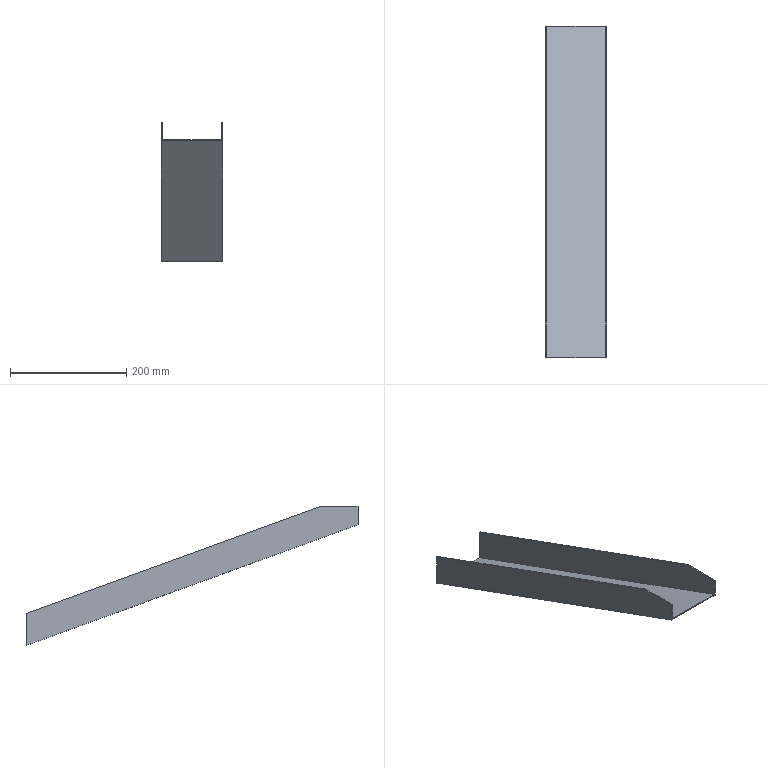Part | NX | features solid 2 | 1 solid | 12 faces | box 105.075 x 570 x 238.942 mm | volume 245403 mm3 | plane 12
STEP:
#1=CARTESIAN_POINT('',(52.538,10.,-231.479));
#2=VERTEX_POINT('',#1);
#3=CARTESIAN_POINT('',(52.538,10.,-200.));
#4=VERTEX_POINT('',#3);
#5=CARTESIAN_POINT('',(52.538,10.,-230.));
#6=DIRECTION('',(0.,0.,1.));
#7=VECTOR('',#6,1000.);
#8=LINE('',#5,#7);
#9=EDGE_CURVE('',#2,#4,#8,.T.);
#10=ORIENTED_EDGE('',*,*,#9,.F.);
#11=CARTESIAN_POINT('',(52.538,580.,-438.942));
#12=VERTEX_POINT('',#11);
#13=CARTESIAN_POINT('',(52.538,11.431,-232.));
#14=DIRECTION('',(0.,-0.9397,0.342));
#15=VECTOR('',#14,1000.);
#16=LINE('',#13,#15);
#17=EDGE_CURVE('',#2,#12,#16,.F.);
#18=ORIENTED_EDGE('',*,*,#17,.T.);
#19=CARTESIAN_POINT('',(52.538,580.,-383.733));
#20=VERTEX_POINT('',#19);
#21=CARTESIAN_POINT('',(52.538,580.,-230.));
#22=DIRECTION('',(0.,0.,1.));
#23=VECTOR('',#22,1000.);
#24=LINE('',#21,#23);
#25=EDGE_CURVE('',#12,#20,#24,.T.);
#26=ORIENTED_EDGE('',*,*,#25,.T.);
#27=CARTESIAN_POINT('',(52.538,75.196,-200.));
#28=VERTEX_POINT('',#27);
#29=CARTESIAN_POINT('',(52.538,28.532,-183.015));
#30=DIRECTION('',(0.,0.9397,-0.342));
#31=VECTOR('',#30,1000.);
#32=LINE('',#29,#31);
#33=EDGE_CURVE('',#28,#20,#32,.T.);
#34=ORIENTED_EDGE('',*,*,#33,.F.);
#35=CARTESIAN_POINT('',(52.538,380.,-200.));
#36=DIRECTION('',(0.,-1.,0.));
#37=VECTOR('',#36,1000.);
#38=LINE('',#35,#37);
#39=EDGE_CURVE('',#28,#4,#38,.T.);
#40=ORIENTED_EDGE('',*,*,#39,.T.);
#41=EDGE_LOOP('',(#10,#18,#26,#34,#40));
#42=FACE_BOUND('',#41,.T.);
#43=CARTESIAN_POINT('',(52.538,11.431,-230.));
#44=DIRECTION('',(-1.,0.,0.));
#45=DIRECTION('',(0.,0.,-1.));
#46=AXIS2_PLACEMENT_3D('',#43,#44,#45);
#47=PLANE('',#46);
#48=ADVANCED_FACE('',(#42),#47,.F.);
#49=CARTESIAN_POINT('',(50.538,10.,-200.));
#50=VERTEX_POINT('',#49);
#51=CARTESIAN_POINT('',(50.538,10.,-229.351));
#52=VERTEX_POINT('',#51);
#53=CARTESIAN_POINT('',(50.538,10.,-183.015));
#54=DIRECTION('',(0.,0.,-1.));
#55=VECTOR('',#54,1000.);
#56=LINE('',#53,#55);
#57=EDGE_CURVE('',#50,#52,#56,.T.);
#58=ORIENTED_EDGE('',*,*,#57,.F.);
#59=CARTESIAN_POINT('',(50.538,75.196,-200.));
#60=VERTEX_POINT('',#59);
#61=CARTESIAN_POINT('',(50.538,380.,-200.));
#62=DIRECTION('',(0.,1.,0.));
#63=VECTOR('',#62,1000.);
#64=LINE('',#61,#63);
#65=EDGE_CURVE('',#50,#60,#64,.T.);
#66=ORIENTED_EDGE('',*,*,#65,.T.);
#67=CARTESIAN_POINT('',(50.538,580.,-383.733));
#68=VERTEX_POINT('',#67);
#69=CARTESIAN_POINT('',(50.538,28.532,-183.015));
#70=DIRECTION('',(0.,0.9397,-0.342));
#71=VECTOR('',#70,1000.);
#72=LINE('',#69,#71);
#73=EDGE_CURVE('',#60,#68,#72,.T.);
#74=ORIENTED_EDGE('',*,*,#73,.T.);
#75=CARTESIAN_POINT('',(50.538,580.,-436.814));
#76=VERTEX_POINT('',#75);
#77=CARTESIAN_POINT('',(50.538,580.,-183.015));
#78=DIRECTION('',(0.,0.,-1.));
#79=VECTOR('',#78,1000.);
#80=LINE('',#77,#79);
#81=EDGE_CURVE('',#68,#76,#80,.T.);
#82=ORIENTED_EDGE('',*,*,#81,.T.);
#83=CARTESIAN_POINT('',(50.538,12.115,-230.121));
#84=DIRECTION('',(0.,-0.9397,0.342));
#85=VECTOR('',#84,1000.);
#86=LINE('',#83,#85);
#87=EDGE_CURVE('',#52,#76,#86,.F.);
#88=ORIENTED_EDGE('',*,*,#87,.F.);
#89=EDGE_LOOP('',(#58,#66,#74,#82,#88));
#90=FACE_BOUND('',#89,.T.);
#91=CARTESIAN_POINT('',(50.538,28.532,-183.015));
#92=DIRECTION('',(1.,0.,0.));
#93=DIRECTION('',(0.,0.,1.));
#94=AXIS2_PLACEMENT_3D('',#91,#92,#93);
#95=PLANE('',#94);
#96=ADVANCED_FACE('',(#90),#95,.F.);
#97=CARTESIAN_POINT('',(-50.538,10.,-229.351));
#98=VERTEX_POINT('',#97);
#99=CARTESIAN_POINT('',(42.538,10.,-229.351));
#100=DIRECTION('',(1.,0.,0.));
#101=VECTOR('',#100,1000.);
#102=LINE('',#99,#101);
#103=EDGE_CURVE('',#52,#98,#102,.F.);
#104=ORIENTED_EDGE('',*,*,#103,.F.);
#105=ORIENTED_EDGE('',*,*,#87,.T.);
#106=CARTESIAN_POINT('',(-50.538,580.,-436.814));
#107=VERTEX_POINT('',#106);
#108=CARTESIAN_POINT('',(42.538,580.,-436.814));
#109=DIRECTION('',(1.,0.,0.));
#110=VECTOR('',#109,1000.);
#111=LINE('',#108,#110);
#112=EDGE_CURVE('',#76,#107,#111,.F.);
#113=ORIENTED_EDGE('',*,*,#112,.T.);
#114=CARTESIAN_POINT('',(-50.538,12.115,-230.121));
#115=DIRECTION('',(0.,-0.9397,0.342));
#116=VECTOR('',#115,1000.);
#117=LINE('',#114,#116);
#118=EDGE_CURVE('',#98,#107,#117,.F.);
#119=ORIENTED_EDGE('',*,*,#118,.F.);
#120=EDGE_LOOP('',(#104,#105,#113,#119));
#121=FACE_BOUND('',#120,.T.);
#122=CARTESIAN_POINT('',(42.538,12.115,-230.121));
#123=DIRECTION('',(0.,0.342,0.9397));
#124=DIRECTION('',(0.,0.9397,-0.342));
#125=AXIS2_PLACEMENT_3D('',#122,#123,#124);
#126=PLANE('',#125);
#127=ADVANCED_FACE('',(#121),#126,.T.);
#128=ORIENTED_EDGE('',*,*,#17,.F.);
#129=CARTESIAN_POINT('',(-52.538,10.,-231.479));
#130=VERTEX_POINT('',#129);
#131=CARTESIAN_POINT('',(42.538,10.,-231.479));
#132=DIRECTION('',(1.,0.,0.));
#133=VECTOR('',#132,1000.);
#134=LINE('',#131,#133);
#135=EDGE_CURVE('',#2,#130,#134,.F.);
#136=ORIENTED_EDGE('',*,*,#135,.T.);
#137=CARTESIAN_POINT('',(-52.538,580.,-438.942));
#138=VERTEX_POINT('',#137);
#139=CARTESIAN_POINT('',(-52.538,11.431,-232.));
#140=DIRECTION('',(0.,-0.9397,0.342));
#141=VECTOR('',#140,1000.);
#142=LINE('',#139,#141);
#143=EDGE_CURVE('',#130,#138,#142,.F.);
#144=ORIENTED_EDGE('',*,*,#143,.T.);
#145=CARTESIAN_POINT('',(42.538,580.,-438.942));
#146=DIRECTION('',(1.,0.,0.));
#147=VECTOR('',#146,1000.);
#148=LINE('',#145,#147);
#149=EDGE_CURVE('',#12,#138,#148,.F.);
#150=ORIENTED_EDGE('',*,*,#149,.F.);
#151=EDGE_LOOP('',(#128,#136,#144,#150));
#152=FACE_BOUND('',#151,.T.);
#153=CARTESIAN_POINT('',(42.538,11.431,-232.));
#154=DIRECTION('',(0.,0.342,0.9397));
#155=DIRECTION('',(0.,0.9397,-0.342));
#156=AXIS2_PLACEMENT_3D('',#153,#154,#155);
#157=PLANE('',#156);
#158=ADVANCED_FACE('',(#152),#157,.F.);
#159=ORIENTED_EDGE('',*,*,#65,.F.);
#160=CARTESIAN_POINT('',(-35.,10.,-200.));
#161=DIRECTION('',(1.,0.,0.));
#162=VECTOR('',#161,1000.);
#163=LINE('',#160,#162);
#164=EDGE_CURVE('',#50,#4,#163,.T.);
#165=ORIENTED_EDGE('',*,*,#164,.T.);
#166=ORIENTED_EDGE('',*,*,#39,.F.);
#167=CARTESIAN_POINT('',(-35.,75.196,-200.));
#168=DIRECTION('',(-1.,0.,0.));
#169=VECTOR('',#168,1000.);
#170=LINE('',#167,#169);
#171=EDGE_CURVE('',#28,#60,#170,.T.);
#172=ORIENTED_EDGE('',*,*,#171,.T.);
#173=EDGE_LOOP('',(#159,#165,#166,#172));
#174=FACE_BOUND('',#173,.T.);
#175=CARTESIAN_POINT('',(-35.,380.,-200.));
#176=DIRECTION('',(0.,0.,1.));
#177=DIRECTION('',(-1.,0.,0.));
#178=AXIS2_PLACEMENT_3D('',#175,#176,#177);
#179=PLANE('',#178);
#180=ADVANCED_FACE('',(#174),#179,.T.);
#181=CARTESIAN_POINT('',(-52.538,10.,-200.));
#182=VERTEX_POINT('',#181);
#183=CARTESIAN_POINT('',(-52.538,10.,-230.));
#184=DIRECTION('',(0.,0.,-1.));
#185=VECTOR('',#184,1000.);
#186=LINE('',#183,#185);
#187=EDGE_CURVE('',#182,#130,#186,.T.);
#188=ORIENTED_EDGE('',*,*,#187,.F.);
#189=CARTESIAN_POINT('',(-52.538,75.196,-200.));
#190=VERTEX_POINT('',#189);
#191=CARTESIAN_POINT('',(-52.538,11.431,-200.));
#192=DIRECTION('',(0.,-1.,0.));
#193=VECTOR('',#192,1000.);
#194=LINE('',#191,#193);
#195=EDGE_CURVE('',#190,#182,#194,.T.);
#196=ORIENTED_EDGE('',*,*,#195,.F.);
#197=CARTESIAN_POINT('',(-52.538,580.,-383.733));
#198=VERTEX_POINT('',#197);
#199=CARTESIAN_POINT('',(-52.538,28.532,-183.015));
#200=DIRECTION('',(0.,0.9397,-0.342));
#201=VECTOR('',#200,1000.);
#202=LINE('',#199,#201);
#203=EDGE_CURVE('',#190,#198,#202,.T.);
#204=ORIENTED_EDGE('',*,*,#203,.T.);
#205=CARTESIAN_POINT('',(-52.538,580.,-405.));
#206=DIRECTION('',(0.,0.,1.));
#207=VECTOR('',#206,1000.);
#208=LINE('',#205,#207);
#209=EDGE_CURVE('',#138,#198,#208,.T.);
#210=ORIENTED_EDGE('',*,*,#209,.F.);
#211=ORIENTED_EDGE('',*,*,#143,.F.);
#212=EDGE_LOOP('',(#188,#196,#204,#210,#211));
#213=FACE_BOUND('',#212,.T.);
#214=CARTESIAN_POINT('',(-52.538,11.431,-230.));
#215=DIRECTION('',(1.,0.,0.));
#216=DIRECTION('',(0.,0.,-1.));
#217=AXIS2_PLACEMENT_3D('',#214,#215,#216);
#218=PLANE('',#217);
#219=ADVANCED_FACE('',(#213),#218,.F.);
#220=CARTESIAN_POINT('',(-50.538,10.,-200.));
#221=VERTEX_POINT('',#220);
#222=CARTESIAN_POINT('',(-50.538,10.,-183.015));
#223=DIRECTION('',(0.,0.,1.));
#224=VECTOR('',#223,1000.);
#225=LINE('',#222,#224);
#226=EDGE_CURVE('',#98,#221,#225,.T.);
#227=ORIENTED_EDGE('',*,*,#226,.F.);
#228=ORIENTED_EDGE('',*,*,#118,.T.);
#229=CARTESIAN_POINT('',(-50.538,580.,-383.733));
#230=VERTEX_POINT('',#229);
#231=CARTESIAN_POINT('',(-50.538,580.,-405.));
#232=DIRECTION('',(0.,0.,-1.));
#233=VECTOR('',#232,1000.);
#234=LINE('',#231,#233);
#235=EDGE_CURVE('',#230,#107,#234,.T.);
#236=ORIENTED_EDGE('',*,*,#235,.F.);
#237=CARTESIAN_POINT('',(-50.538,75.196,-200.));
#238=VERTEX_POINT('',#237);
#239=CARTESIAN_POINT('',(-50.538,28.532,-183.015));
#240=DIRECTION('',(0.,0.9397,-0.342));
#241=VECTOR('',#240,1000.);
#242=LINE('',#239,#241);
#243=EDGE_CURVE('',#238,#230,#242,.T.);
#244=ORIENTED_EDGE('',*,*,#243,.F.);
#245=CARTESIAN_POINT('',(-50.538,28.532,-200.));
#246=DIRECTION('',(0.,1.,0.));
#247=VECTOR('',#246,1000.);
#248=LINE('',#245,#247);
#249=EDGE_CURVE('',#221,#238,#248,.T.);
#250=ORIENTED_EDGE('',*,*,#249,.F.);
#251=EDGE_LOOP('',(#227,#228,#236,#244,#250));
#252=FACE_BOUND('',#251,.T.);
#253=CARTESIAN_POINT('',(-50.538,28.532,-183.015));
#254=DIRECTION('',(-1.,0.,0.));
#255=DIRECTION('',(0.,0.,1.));
#256=AXIS2_PLACEMENT_3D('',#253,#254,#255);
#257=PLANE('',#256);
#258=ADVANCED_FACE('',(#252),#257,.F.);
#259=ORIENTED_EDGE('',*,*,#195,.T.);
#260=CARTESIAN_POINT('',(35.,10.,-200.));
#261=DIRECTION('',(1.,0.,0.));
#262=VECTOR('',#261,1000.);
#263=LINE('',#260,#262);
#264=EDGE_CURVE('',#182,#221,#263,.T.);
#265=ORIENTED_EDGE('',*,*,#264,.T.);
#266=ORIENTED_EDGE('',*,*,#249,.T.);
#267=CARTESIAN_POINT('',(-52.538,75.196,-200.));
#268=DIRECTION('',(1.,0.,0.));
#269=VECTOR('',#268,1000.);
#270=LINE('',#267,#269);
#271=EDGE_CURVE('',#190,#238,#270,.T.);
#272=ORIENTED_EDGE('',*,*,#271,.F.);
#273=EDGE_LOOP('',(#259,#265,#266,#272));
#274=FACE_BOUND('',#273,.T.);
#275=CARTESIAN_POINT('',(35.,380.,-200.));
#276=DIRECTION('',(0.,0.,1.));
#277=DIRECTION('',(1.,0.,0.));
#278=AXIS2_PLACEMENT_3D('',#275,#276,#277);
#279=PLANE('',#278);
#280=ADVANCED_FACE('',(#274),#279,.T.);
#281=ORIENTED_EDGE('',*,*,#33,.T.);
#282=CARTESIAN_POINT('',(330.,580.,-383.733));
#283=DIRECTION('',(-1.,0.,0.));
#284=VECTOR('',#283,1000.);
#285=LINE('',#282,#284);
#286=EDGE_CURVE('',#20,#68,#285,.T.);
#287=ORIENTED_EDGE('',*,*,#286,.T.);
#288=ORIENTED_EDGE('',*,*,#73,.F.);
#289=ORIENTED_EDGE('',*,*,#171,.F.);
#290=EDGE_LOOP('',(#281,#287,#288,#289));
#291=FACE_BOUND('',#290,.T.);
#292=CARTESIAN_POINT('',(52.538,28.532,-183.015));
#293=DIRECTION('',(0.,0.342,0.9397));
#294=DIRECTION('',(0.,0.9397,-0.342));
#295=AXIS2_PLACEMENT_3D('',#292,#293,#294);
#296=PLANE('',#295);
#297=ADVANCED_FACE('',(#291),#296,.T.);
#298=ORIENTED_EDGE('',*,*,#25,.F.);
#299=ORIENTED_EDGE('',*,*,#149,.T.);
#300=ORIENTED_EDGE('',*,*,#209,.T.);
#301=CARTESIAN_POINT('',(-52.538,580.,-383.733));
#302=DIRECTION('',(1.,0.,0.));
#303=VECTOR('',#302,1000.);
#304=LINE('',#301,#303);
#305=EDGE_CURVE('',#198,#230,#304,.T.);
#306=ORIENTED_EDGE('',*,*,#305,.T.);
#307=ORIENTED_EDGE('',*,*,#235,.T.);
#308=ORIENTED_EDGE('',*,*,#112,.F.);
#309=ORIENTED_EDGE('',*,*,#81,.F.);
#310=ORIENTED_EDGE('',*,*,#286,.F.);
#311=EDGE_LOOP('',(#298,#299,#300,#306,#307,#308,#309,#310));
#312=FACE_BOUND('',#311,.T.);
#313=CARTESIAN_POINT('',(330.,580.,-405.));
#314=DIRECTION('',(0.,-1.,0.));
#315=DIRECTION('',(1.,0.,0.));
#316=AXIS2_PLACEMENT_3D('',#313,#314,#315);
#317=PLANE('',#316);
#318=ADVANCED_FACE('',(#312),#317,.F.);
#319=ORIENTED_EDGE('',*,*,#203,.F.);
#320=ORIENTED_EDGE('',*,*,#271,.T.);
#321=ORIENTED_EDGE('',*,*,#243,.T.);
#322=ORIENTED_EDGE('',*,*,#305,.F.);
#323=EDGE_LOOP('',(#319,#320,#321,#322));
#324=FACE_BOUND('',#323,.T.);
#325=CARTESIAN_POINT('',(-52.538,28.532,-183.015));
#326=DIRECTION('',(0.,0.342,0.9397));
#327=DIRECTION('',(0.,0.9397,-0.342));
#328=AXIS2_PLACEMENT_3D('',#325,#326,#327);
#329=PLANE('',#328);
#330=ADVANCED_FACE('',(#324),#329,.T.);
#331=ORIENTED_EDGE('',*,*,#164,.F.);
#332=ORIENTED_EDGE('',*,*,#57,.T.);
#333=ORIENTED_EDGE('',*,*,#103,.T.);
#334=ORIENTED_EDGE('',*,*,#226,.T.);
#335=ORIENTED_EDGE('',*,*,#264,.F.);
#336=ORIENTED_EDGE('',*,*,#187,.T.);
#337=ORIENTED_EDGE('',*,*,#135,.F.);
#338=ORIENTED_EDGE('',*,*,#9,.T.);
#339=EDGE_LOOP('',(#331,#332,#333,#334,#335,#336,#337,#338));
#340=FACE_BOUND('',#339,.T.);
#341=CARTESIAN_POINT('',(-210.,10.,0.));
#342=DIRECTION('',(0.,-1.,0.));
#343=DIRECTION('',(0.,0.,-1.));
#344=AXIS2_PLACEMENT_3D('',#341,#342,#343);
#345=PLANE('',#344);
#346=ADVANCED_FACE('',(#340),#345,.T.);
#347=CLOSED_SHELL('',(#48,#96,#127,#158,#180,#219,#258,#280,#297,#318,#330,#346));
#348=MANIFOLD_SOLID_BREP('',#347);
#349=(LENGTH_UNIT()NAMED_UNIT(*)SI_UNIT(.MILLI.,.METRE.));
#350=UNCERTAINTY_MEASURE_WITH_UNIT(LENGTH_MEASURE(0.00001),#349,'','');
#351=(NAMED_UNIT(*)PLANE_ANGLE_UNIT()SI_UNIT($,.RADIAN.));
#352=(NAMED_UNIT(*)SI_UNIT($,.STERADIAN.)SOLID_ANGLE_UNIT());
#353=(GEOMETRIC_REPRESENTATION_CONTEXT(3)GLOBAL_UNCERTAINTY_ASSIGNED_CONTEXT((#350))GLOBAL_UNIT_ASSIGNED_CONTEXT((#349,#351,#352))REPRESENTATION_CONTEXT('',''));
#354=ADVANCED_BREP_SHAPE_REPRESENTATION('',(#348),#353);